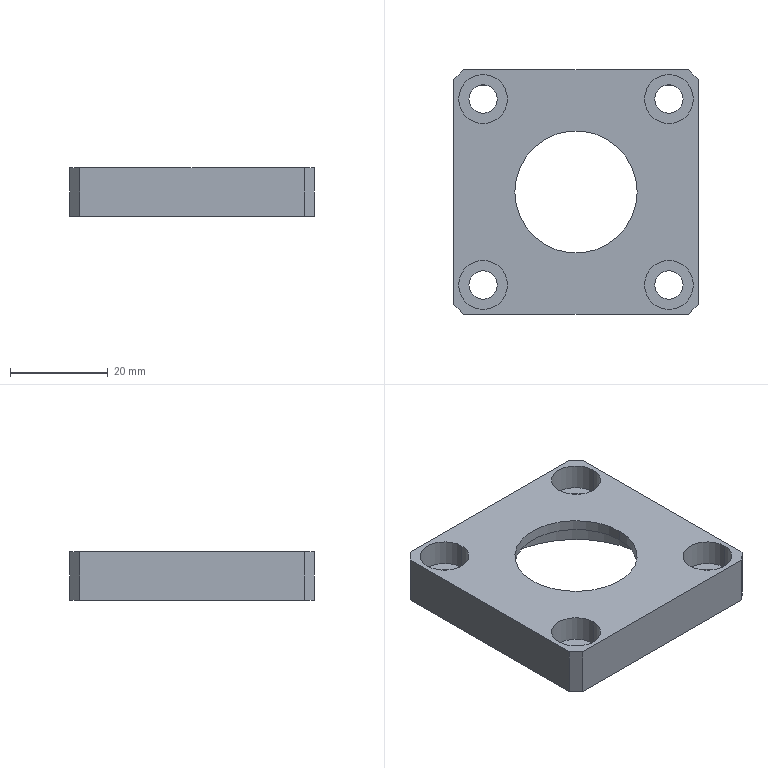Part | SolidWorks | features ICE 2, Chamfer 1, Extrusion 1, HoleWzd 1 | 1 solid | 35 faces | box 50 x 50 x 10 mm | volume 11856 mm3 | cylinder 20 | plane 15 | commonest cylinder face diameters 5.8 x8 10 x8 25 x2 40 x2
STEP:
#1=CARTESIAN_POINT('',(-12.5,0.,2.8));
#2=VERTEX_POINT('',#1);
#3=CARTESIAN_POINT('',(12.5,0.,2.8));
#4=VERTEX_POINT('',#3);
#5=CARTESIAN_POINT('',(0.,0.,2.8));
#6=DIRECTION('',(0.,0.,1.));
#7=DIRECTION('',(1.,0.,0.));
#8=AXIS2_PLACEMENT_3D('',#5,#6,#7);
#9=CIRCLE('',#8,12.5);
#10=EDGE_CURVE('',#2,#4,#9,.T.);
#11=ORIENTED_EDGE('',*,*,#10,.F.);
#12=CARTESIAN_POINT('',(-12.5,0.,5.));
#13=VERTEX_POINT('',#12);
#14=CARTESIAN_POINT('',(-12.5,0.,2.8));
#15=DIRECTION('',(0.,0.,1.));
#16=VECTOR('',#15,1000.);
#17=LINE('',#14,#16);
#18=EDGE_CURVE('',#2,#13,#17,.T.);
#19=ORIENTED_EDGE('',*,*,#18,.T.);
#20=CARTESIAN_POINT('',(12.5,0.,5.));
#21=VERTEX_POINT('',#20);
#22=CARTESIAN_POINT('',(0.,0.,5.));
#23=DIRECTION('',(0.,0.,1.));
#24=DIRECTION('',(1.,0.,0.));
#25=AXIS2_PLACEMENT_3D('',#22,#23,#24);
#26=CIRCLE('',#25,12.5);
#27=EDGE_CURVE('',#13,#21,#26,.T.);
#28=ORIENTED_EDGE('',*,*,#27,.T.);
#29=CARTESIAN_POINT('',(12.5,0.,2.8));
#30=DIRECTION('',(0.,0.,1.));
#31=VECTOR('',#30,1000.);
#32=LINE('',#29,#31);
#33=EDGE_CURVE('',#4,#21,#32,.T.);
#34=ORIENTED_EDGE('',*,*,#33,.F.);
#35=EDGE_LOOP('',(#11,#19,#28,#34));
#36=FACE_OUTER_BOUND('',#35,.T.);
#37=CARTESIAN_POINT('',(0.,0.,2.8));
#38=DIRECTION('',(0.,0.,1.));
#39=DIRECTION('',(1.,0.,0.));
#40=AXIS2_PLACEMENT_3D('',#37,#38,#39);
#41=CYLINDRICAL_SURFACE('',#40,12.5);
#42=ADVANCED_FACE('',(#36),#41,.F.);
#43=CARTESIAN_POINT('',(-24.,19.,-0.4));
#44=VERTEX_POINT('',#43);
#45=CARTESIAN_POINT('',(-14.,19.,-0.4));
#46=VERTEX_POINT('',#45);
#47=CARTESIAN_POINT('',(-19.,19.,-0.4));
#48=DIRECTION('',(0.,0.,1.));
#49=DIRECTION('',(1.,0.,0.));
#50=AXIS2_PLACEMENT_3D('',#47,#48,#49);
#51=CIRCLE('',#50,5.);
#52=EDGE_CURVE('',#44,#46,#51,.T.);
#53=ORIENTED_EDGE('',*,*,#52,.F.);
#54=CARTESIAN_POINT('',(-24.,19.,5.));
#55=VERTEX_POINT('',#54);
#56=CARTESIAN_POINT('',(-24.,19.,5.));
#57=DIRECTION('',(0.,0.,1.));
#58=VECTOR('',#57,1000.);
#59=LINE('',#56,#58);
#60=EDGE_CURVE('',#44,#55,#59,.T.);
#61=ORIENTED_EDGE('',*,*,#60,.T.);
#62=CARTESIAN_POINT('',(-14.,19.,5.));
#63=VERTEX_POINT('',#62);
#64=CARTESIAN_POINT('',(-19.,19.,5.));
#65=DIRECTION('',(0.,0.,1.));
#66=DIRECTION('',(1.,0.,0.));
#67=AXIS2_PLACEMENT_3D('',#64,#65,#66);
#68=CIRCLE('',#67,5.);
#69=EDGE_CURVE('',#55,#63,#68,.T.);
#70=ORIENTED_EDGE('',*,*,#69,.T.);
#71=CARTESIAN_POINT('',(-14.,19.,5.));
#72=DIRECTION('',(0.,0.,1.));
#73=VECTOR('',#72,1000.);
#74=LINE('',#71,#73);
#75=EDGE_CURVE('',#46,#63,#74,.T.);
#76=ORIENTED_EDGE('',*,*,#75,.F.);
#77=EDGE_LOOP('',(#53,#61,#70,#76));
#78=FACE_OUTER_BOUND('',#77,.T.);
#79=CARTESIAN_POINT('',(-19.,19.,5.));
#80=DIRECTION('',(0.,0.,1.));
#81=DIRECTION('',(1.,0.,0.));
#82=AXIS2_PLACEMENT_3D('',#79,#80,#81);
#83=CYLINDRICAL_SURFACE('',#82,5.);
#84=ADVANCED_FACE('',(#78),#83,.F.);
#85=CARTESIAN_POINT('',(-21.9,19.,-5.));
#86=VERTEX_POINT('',#85);
#87=CARTESIAN_POINT('',(-16.1,19.,-5.));
#88=VERTEX_POINT('',#87);
#89=CARTESIAN_POINT('',(-19.,19.,-5.));
#90=DIRECTION('',(0.,0.,1.));
#91=DIRECTION('',(1.,0.,0.));
#92=AXIS2_PLACEMENT_3D('',#89,#90,#91);
#93=CIRCLE('',#92,2.9);
#94=EDGE_CURVE('',#86,#88,#93,.T.);
#95=ORIENTED_EDGE('',*,*,#94,.F.);
#96=CARTESIAN_POINT('',(-21.9,19.,-0.4));
#97=VERTEX_POINT('',#96);
#98=CARTESIAN_POINT('',(-21.9,19.,5.));
#99=DIRECTION('',(0.,0.,1.));
#100=VECTOR('',#99,1000.);
#101=LINE('',#98,#100);
#102=EDGE_CURVE('',#86,#97,#101,.T.);
#103=ORIENTED_EDGE('',*,*,#102,.T.);
#104=CARTESIAN_POINT('',(-16.1,19.,-0.4));
#105=VERTEX_POINT('',#104);
#106=CARTESIAN_POINT('',(-19.,19.,-0.4));
#107=DIRECTION('',(0.,0.,1.));
#108=DIRECTION('',(1.,0.,0.));
#109=AXIS2_PLACEMENT_3D('',#106,#107,#108);
#110=CIRCLE('',#109,2.9);
#111=EDGE_CURVE('',#97,#105,#110,.T.);
#112=ORIENTED_EDGE('',*,*,#111,.T.);
#113=CARTESIAN_POINT('',(-16.1,19.,5.));
#114=DIRECTION('',(0.,0.,1.));
#115=VECTOR('',#114,1000.);
#116=LINE('',#113,#115);
#117=EDGE_CURVE('',#88,#105,#116,.T.);
#118=ORIENTED_EDGE('',*,*,#117,.F.);
#119=EDGE_LOOP('',(#95,#103,#112,#118));
#120=FACE_OUTER_BOUND('',#119,.T.);
#121=CARTESIAN_POINT('',(-19.,19.,5.));
#122=DIRECTION('',(0.,0.,1.));
#123=DIRECTION('',(1.,0.,0.));
#124=AXIS2_PLACEMENT_3D('',#121,#122,#123);
#125=CYLINDRICAL_SURFACE('',#124,2.9);
#126=ADVANCED_FACE('',(#120),#125,.F.);
#127=CARTESIAN_POINT('',(14.,19.,-0.4));
#128=VERTEX_POINT('',#127);
#129=CARTESIAN_POINT('',(24.,19.,-0.4));
#130=VERTEX_POINT('',#129);
#131=CARTESIAN_POINT('',(19.,19.,-0.4));
#132=DIRECTION('',(0.,0.,1.));
#133=DIRECTION('',(1.,0.,0.));
#134=AXIS2_PLACEMENT_3D('',#131,#132,#133);
#135=CIRCLE('',#134,5.);
#136=EDGE_CURVE('',#128,#130,#135,.T.);
#137=ORIENTED_EDGE('',*,*,#136,.F.);
#138=CARTESIAN_POINT('',(14.,19.,5.));
#139=VERTEX_POINT('',#138);
#140=CARTESIAN_POINT('',(14.,19.,5.));
#141=DIRECTION('',(0.,0.,1.));
#142=VECTOR('',#141,1000.);
#143=LINE('',#140,#142);
#144=EDGE_CURVE('',#128,#139,#143,.T.);
#145=ORIENTED_EDGE('',*,*,#144,.T.);
#146=CARTESIAN_POINT('',(24.,19.,5.));
#147=VERTEX_POINT('',#146);
#148=CARTESIAN_POINT('',(19.,19.,5.));
#149=DIRECTION('',(0.,0.,1.));
#150=DIRECTION('',(1.,0.,0.));
#151=AXIS2_PLACEMENT_3D('',#148,#149,#150);
#152=CIRCLE('',#151,5.);
#153=EDGE_CURVE('',#139,#147,#152,.T.);
#154=ORIENTED_EDGE('',*,*,#153,.T.);
#155=CARTESIAN_POINT('',(24.,19.,5.));
#156=DIRECTION('',(0.,0.,1.));
#157=VECTOR('',#156,1000.);
#158=LINE('',#155,#157);
#159=EDGE_CURVE('',#130,#147,#158,.T.);
#160=ORIENTED_EDGE('',*,*,#159,.F.);
#161=EDGE_LOOP('',(#137,#145,#154,#160));
#162=FACE_OUTER_BOUND('',#161,.T.);
#163=CARTESIAN_POINT('',(19.,19.,5.));
#164=DIRECTION('',(0.,0.,1.));
#165=DIRECTION('',(1.,0.,0.));
#166=AXIS2_PLACEMENT_3D('',#163,#164,#165);
#167=CYLINDRICAL_SURFACE('',#166,5.);
#168=ADVANCED_FACE('',(#162),#167,.F.);
#169=CARTESIAN_POINT('',(16.1,19.,-5.));
#170=VERTEX_POINT('',#169);
#171=CARTESIAN_POINT('',(21.9,19.,-5.));
#172=VERTEX_POINT('',#171);
#173=CARTESIAN_POINT('',(19.,19.,-5.));
#174=DIRECTION('',(0.,0.,1.));
#175=DIRECTION('',(1.,0.,0.));
#176=AXIS2_PLACEMENT_3D('',#173,#174,#175);
#177=CIRCLE('',#176,2.9);
#178=EDGE_CURVE('',#170,#172,#177,.T.);
#179=ORIENTED_EDGE('',*,*,#178,.F.);
#180=CARTESIAN_POINT('',(16.1,19.,-0.4));
#181=VERTEX_POINT('',#180);
#182=CARTESIAN_POINT('',(16.1,19.,5.));
#183=DIRECTION('',(0.,0.,1.));
#184=VECTOR('',#183,1000.);
#185=LINE('',#182,#184);
#186=EDGE_CURVE('',#170,#181,#185,.T.);
#187=ORIENTED_EDGE('',*,*,#186,.T.);
#188=CARTESIAN_POINT('',(21.9,19.,-0.4));
#189=VERTEX_POINT('',#188);
#190=CARTESIAN_POINT('',(19.,19.,-0.4));
#191=DIRECTION('',(0.,0.,1.));
#192=DIRECTION('',(1.,0.,0.));
#193=AXIS2_PLACEMENT_3D('',#190,#191,#192);
#194=CIRCLE('',#193,2.9);
#195=EDGE_CURVE('',#181,#189,#194,.T.);
#196=ORIENTED_EDGE('',*,*,#195,.T.);
#197=CARTESIAN_POINT('',(21.9,19.,5.));
#198=DIRECTION('',(0.,0.,1.));
#199=VECTOR('',#198,1000.);
#200=LINE('',#197,#199);
#201=EDGE_CURVE('',#172,#189,#200,.T.);
#202=ORIENTED_EDGE('',*,*,#201,.F.);
#203=EDGE_LOOP('',(#179,#187,#196,#202));
#204=FACE_OUTER_BOUND('',#203,.T.);
#205=CARTESIAN_POINT('',(19.,19.,5.));
#206=DIRECTION('',(0.,0.,1.));
#207=DIRECTION('',(1.,0.,0.));
#208=AXIS2_PLACEMENT_3D('',#205,#206,#207);
#209=CYLINDRICAL_SURFACE('',#208,2.9);
#210=ADVANCED_FACE('',(#204),#209,.F.);
#211=CARTESIAN_POINT('',(-24.,-19.,-0.4));
#212=VERTEX_POINT('',#211);
#213=CARTESIAN_POINT('',(-14.,-19.,-0.4));
#214=VERTEX_POINT('',#213);
#215=CARTESIAN_POINT('',(-19.,-19.,-0.4));
#216=DIRECTION('',(0.,0.,1.));
#217=DIRECTION('',(1.,0.,0.));
#218=AXIS2_PLACEMENT_3D('',#215,#216,#217);
#219=CIRCLE('',#218,5.);
#220=EDGE_CURVE('',#212,#214,#219,.T.);
#221=ORIENTED_EDGE('',*,*,#220,.F.);
#222=CARTESIAN_POINT('',(-24.,-19.,5.));
#223=VERTEX_POINT('',#222);
#224=CARTESIAN_POINT('',(-24.,-19.,5.));
#225=DIRECTION('',(0.,0.,1.));
#226=VECTOR('',#225,1000.);
#227=LINE('',#224,#226);
#228=EDGE_CURVE('',#212,#223,#227,.T.);
#229=ORIENTED_EDGE('',*,*,#228,.T.);
#230=CARTESIAN_POINT('',(-14.,-19.,5.));
#231=VERTEX_POINT('',#230);
#232=CARTESIAN_POINT('',(-19.,-19.,5.));
#233=DIRECTION('',(0.,0.,1.));
#234=DIRECTION('',(1.,0.,0.));
#235=AXIS2_PLACEMENT_3D('',#232,#233,#234);
#236=CIRCLE('',#235,5.);
#237=EDGE_CURVE('',#223,#231,#236,.T.);
#238=ORIENTED_EDGE('',*,*,#237,.T.);
#239=CARTESIAN_POINT('',(-14.,-19.,5.));
#240=DIRECTION('',(0.,0.,1.));
#241=VECTOR('',#240,1000.);
#242=LINE('',#239,#241);
#243=EDGE_CURVE('',#214,#231,#242,.T.);
#244=ORIENTED_EDGE('',*,*,#243,.F.);
#245=EDGE_LOOP('',(#221,#229,#238,#244));
#246=FACE_OUTER_BOUND('',#245,.T.);
#247=CARTESIAN_POINT('',(-19.,-19.,5.));
#248=DIRECTION('',(0.,0.,1.));
#249=DIRECTION('',(1.,0.,0.));
#250=AXIS2_PLACEMENT_3D('',#247,#248,#249);
#251=CYLINDRICAL_SURFACE('',#250,5.);
#252=ADVANCED_FACE('',(#246),#251,.F.);
#253=CARTESIAN_POINT('',(-21.9,-19.,-5.));
#254=VERTEX_POINT('',#253);
#255=CARTESIAN_POINT('',(-16.1,-19.,-5.));
#256=VERTEX_POINT('',#255);
#257=CARTESIAN_POINT('',(-19.,-19.,-5.));
#258=DIRECTION('',(0.,0.,1.));
#259=DIRECTION('',(1.,0.,0.));
#260=AXIS2_PLACEMENT_3D('',#257,#258,#259);
#261=CIRCLE('',#260,2.9);
#262=EDGE_CURVE('',#254,#256,#261,.T.);
#263=ORIENTED_EDGE('',*,*,#262,.F.);
#264=CARTESIAN_POINT('',(-21.9,-19.,-0.4));
#265=VERTEX_POINT('',#264);
#266=CARTESIAN_POINT('',(-21.9,-19.,5.));
#267=DIRECTION('',(0.,0.,1.));
#268=VECTOR('',#267,1000.);
#269=LINE('',#266,#268);
#270=EDGE_CURVE('',#254,#265,#269,.T.);
#271=ORIENTED_EDGE('',*,*,#270,.T.);
#272=CARTESIAN_POINT('',(-16.1,-19.,-0.4));
#273=VERTEX_POINT('',#272);
#274=CARTESIAN_POINT('',(-19.,-19.,-0.4));
#275=DIRECTION('',(0.,0.,1.));
#276=DIRECTION('',(1.,0.,0.));
#277=AXIS2_PLACEMENT_3D('',#274,#275,#276);
#278=CIRCLE('',#277,2.9);
#279=EDGE_CURVE('',#265,#273,#278,.T.);
#280=ORIENTED_EDGE('',*,*,#279,.T.);
#281=CARTESIAN_POINT('',(-16.1,-19.,5.));
#282=DIRECTION('',(0.,0.,1.));
#283=VECTOR('',#282,1000.);
#284=LINE('',#281,#283);
#285=EDGE_CURVE('',#256,#273,#284,.T.);
#286=ORIENTED_EDGE('',*,*,#285,.F.);
#287=EDGE_LOOP('',(#263,#271,#280,#286));
#288=FACE_OUTER_BOUND('',#287,.T.);
#289=CARTESIAN_POINT('',(-19.,-19.,5.));
#290=DIRECTION('',(0.,0.,1.));
#291=DIRECTION('',(1.,0.,0.));
#292=AXIS2_PLACEMENT_3D('',#289,#290,#291);
#293=CYLINDRICAL_SURFACE('',#292,2.9);
#294=ADVANCED_FACE('',(#288),#293,.F.);
#295=CARTESIAN_POINT('',(14.,-19.,-0.4));
#296=VERTEX_POINT('',#295);
#297=CARTESIAN_POINT('',(24.,-19.,-0.4));
#298=VERTEX_POINT('',#297);
#299=CARTESIAN_POINT('',(19.,-19.,-0.4));
#300=DIRECTION('',(0.,0.,1.));
#301=DIRECTION('',(1.,0.,0.));
#302=AXIS2_PLACEMENT_3D('',#299,#300,#301);
#303=CIRCLE('',#302,5.);
#304=EDGE_CURVE('',#296,#298,#303,.T.);
#305=ORIENTED_EDGE('',*,*,#304,.F.);
#306=CARTESIAN_POINT('',(14.,-19.,5.));
#307=VERTEX_POINT('',#306);
#308=CARTESIAN_POINT('',(14.,-19.,5.));
#309=DIRECTION('',(0.,0.,1.));
#310=VECTOR('',#309,1000.);
#311=LINE('',#308,#310);
#312=EDGE_CURVE('',#296,#307,#311,.T.);
#313=ORIENTED_EDGE('',*,*,#312,.T.);
#314=CARTESIAN_POINT('',(24.,-19.,5.));
#315=VERTEX_POINT('',#314);
#316=CARTESIAN_POINT('',(19.,-19.,5.));
#317=DIRECTION('',(0.,0.,1.));
#318=DIRECTION('',(1.,0.,0.));
#319=AXIS2_PLACEMENT_3D('',#316,#317,#318);
#320=CIRCLE('',#319,5.);
#321=EDGE_CURVE('',#307,#315,#320,.T.);
#322=ORIENTED_EDGE('',*,*,#321,.T.);
#323=CARTESIAN_POINT('',(24.,-19.,5.));
#324=DIRECTION('',(0.,0.,1.));
#325=VECTOR('',#324,1000.);
#326=LINE('',#323,#325);
#327=EDGE_CURVE('',#298,#315,#326,.T.);
#328=ORIENTED_EDGE('',*,*,#327,.F.);
#329=EDGE_LOOP('',(#305,#313,#322,#328));
#330=FACE_OUTER_BOUND('',#329,.T.);
#331=CARTESIAN_POINT('',(19.,-19.,5.));
#332=DIRECTION('',(0.,0.,1.));
#333=DIRECTION('',(1.,0.,0.));
#334=AXIS2_PLACEMENT_3D('',#331,#332,#333);
#335=CYLINDRICAL_SURFACE('',#334,5.);
#336=ADVANCED_FACE('',(#330),#335,.F.);
#337=CARTESIAN_POINT('',(16.1,-19.,-5.));
#338=VERTEX_POINT('',#337);
#339=CARTESIAN_POINT('',(21.9,-19.,-5.));
#340=VERTEX_POINT('',#339);
#341=CARTESIAN_POINT('',(19.,-19.,-5.));
#342=DIRECTION('',(0.,0.,1.));
#343=DIRECTION('',(1.,0.,0.));
#344=AXIS2_PLACEMENT_3D('',#341,#342,#343);
#345=CIRCLE('',#344,2.9);
#346=EDGE_CURVE('',#338,#340,#345,.T.);
#347=ORIENTED_EDGE('',*,*,#346,.F.);
#348=CARTESIAN_POINT('',(16.1,-19.,-0.4));
#349=VERTEX_POINT('',#348);
#350=CARTESIAN_POINT('',(16.1,-19.,5.));
#351=DIRECTION('',(0.,0.,1.));
#352=VECTOR('',#351,1000.);
#353=LINE('',#350,#352);
#354=EDGE_CURVE('',#338,#349,#353,.T.);
#355=ORIENTED_EDGE('',*,*,#354,.T.);
#356=CARTESIAN_POINT('',(21.9,-19.,-0.4));
#357=VERTEX_POINT('',#356);
#358=CARTESIAN_POINT('',(19.,-19.,-0.4));
#359=DIRECTION('',(0.,0.,1.));
#360=DIRECTION('',(1.,0.,0.));
#361=AXIS2_PLACEMENT_3D('',#358,#359,#360);
#362=CIRCLE('',#361,2.9);
#363=EDGE_CURVE('',#349,#357,#362,.T.);
#364=ORIENTED_EDGE('',*,*,#363,.T.);
#365=CARTESIAN_POINT('',(21.9,-19.,5.));
#366=DIRECTION('',(0.,0.,1.));
#367=VECTOR('',#366,1000.);
#368=LINE('',#365,#367);
#369=EDGE_CURVE('',#340,#357,#368,.T.);
#370=ORIENTED_EDGE('',*,*,#369,.F.);
#371=EDGE_LOOP('',(#347,#355,#364,#370));
#372=FACE_OUTER_BOUND('',#371,.T.);
#373=CARTESIAN_POINT('',(19.,-19.,5.));
#374=DIRECTION('',(0.,0.,1.));
#375=DIRECTION('',(1.,0.,0.));
#376=AXIS2_PLACEMENT_3D('',#373,#374,#375);
#377=CYLINDRICAL_SURFACE('',#376,2.9);
#378=ADVANCED_FACE('',(#372),#377,.F.);
#379=CARTESIAN_POINT('',(-20.,0.,-5.));
#380=VERTEX_POINT('',#379);
#381=CARTESIAN_POINT('',(20.,0.,-5.));
#382=VERTEX_POINT('',#381);
#383=CARTESIAN_POINT('',(0.,0.,-5.));
#384=DIRECTION('',(0.,0.,1.));
#385=DIRECTION('',(1.,0.,0.));
#386=AXIS2_PLACEMENT_3D('',#383,#384,#385);
#387=CIRCLE('',#386,20.);
#388=EDGE_CURVE('',#380,#382,#387,.T.);
#389=ORIENTED_EDGE('',*,*,#388,.F.);
#390=CARTESIAN_POINT('',(-20.,0.,2.8));
#391=VERTEX_POINT('',#390);
#392=CARTESIAN_POINT('',(-20.,0.,-5.));
#393=DIRECTION('',(0.,0.,1.));
#394=VECTOR('',#393,1000.);
#395=LINE('',#392,#394);
#396=EDGE_CURVE('',#380,#391,#395,.T.);
#397=ORIENTED_EDGE('',*,*,#396,.T.);
#398=CARTESIAN_POINT('',(20.,0.,2.8));
#399=VERTEX_POINT('',#398);
#400=CARTESIAN_POINT('',(0.,0.,2.8));
#401=DIRECTION('',(0.,0.,-1.));
#402=DIRECTION('',(1.,0.,0.));
#403=AXIS2_PLACEMENT_3D('',#400,#401,#402);
#404=CIRCLE('',#403,20.);
#405=EDGE_CURVE('',#399,#391,#404,.T.);
#406=ORIENTED_EDGE('',*,*,#405,.F.);
#407=CARTESIAN_POINT('',(20.,0.,-5.));
#408=DIRECTION('',(0.,0.,1.));
#409=VECTOR('',#408,1000.);
#410=LINE('',#407,#409);
#411=EDGE_CURVE('',#382,#399,#410,.T.);
#412=ORIENTED_EDGE('',*,*,#411,.F.);
#413=EDGE_LOOP('',(#389,#397,#406,#412));
#414=FACE_OUTER_BOUND('',#413,.T.);
#415=CARTESIAN_POINT('',(0.,0.,-5.));
#416=DIRECTION('',(0.,0.,1.));
#417=DIRECTION('',(1.,0.,0.));
#418=AXIS2_PLACEMENT_3D('',#415,#416,#417);
#419=CYLINDRICAL_SURFACE('',#418,20.);
#420=ADVANCED_FACE('',(#414),#419,.F.);
#421=ORIENTED_EDGE('',*,*,#396,.F.);
#422=CARTESIAN_POINT('',(0.,0.,-5.));
#423=DIRECTION('',(0.,0.,1.));
#424=DIRECTION('',(1.,0.,0.));
#425=AXIS2_PLACEMENT_3D('',#422,#423,#424);
#426=CIRCLE('',#425,20.);
#427=EDGE_CURVE('',#382,#380,#426,.T.);
#428=ORIENTED_EDGE('',*,*,#427,.F.);
#429=ORIENTED_EDGE('',*,*,#411,.T.);
#430=CARTESIAN_POINT('',(0.,0.,2.8));
#431=DIRECTION('',(0.,0.,-1.));
#432=DIRECTION('',(1.,0.,0.));
#433=AXIS2_PLACEMENT_3D('',#430,#431,#432);
#434=CIRCLE('',#433,20.);
#435=EDGE_CURVE('',#391,#399,#434,.T.);
#436=ORIENTED_EDGE('',*,*,#435,.F.);
#437=EDGE_LOOP('',(#421,#428,#429,#436));
#438=FACE_OUTER_BOUND('',#437,.T.);
#439=CARTESIAN_POINT('',(0.,0.,-5.));
#440=DIRECTION('',(0.,0.,1.));
#441=DIRECTION('',(1.,0.,0.));
#442=AXIS2_PLACEMENT_3D('',#439,#440,#441);
#443=CYLINDRICAL_SURFACE('',#442,20.);
#444=ADVANCED_FACE('',(#438),#443,.F.);
#445=CARTESIAN_POINT('',(25.,-23.,5.));
#446=VERTEX_POINT('',#445);
#447=CARTESIAN_POINT('',(25.,23.,5.));
#448=VERTEX_POINT('',#447);
#449=CARTESIAN_POINT('',(25.,-25.,5.));
#450=DIRECTION('',(0.,1.,0.));
#451=VECTOR('',#450,1000.);
#452=LINE('',#449,#451);
#453=EDGE_CURVE('',#446,#448,#452,.T.);
#454=ORIENTED_EDGE('',*,*,#453,.F.);
#455=CARTESIAN_POINT('',(25.,-23.,-5.));
#456=VERTEX_POINT('',#455);
#457=CARTESIAN_POINT('',(25.,-23.,5.));
#458=DIRECTION('',(0.,0.,-1.));
#459=VECTOR('',#458,1000.);
#460=LINE('',#457,#459);
#461=EDGE_CURVE('',#446,#456,#460,.T.);
#462=ORIENTED_EDGE('',*,*,#461,.T.);
#463=CARTESIAN_POINT('',(25.,23.,-5.));
#464=VERTEX_POINT('',#463);
#465=CARTESIAN_POINT('',(25.,-25.,-5.));
#466=DIRECTION('',(0.,1.,0.));
#467=VECTOR('',#466,1000.);
#468=LINE('',#465,#467);
#469=EDGE_CURVE('',#456,#464,#468,.T.);
#470=ORIENTED_EDGE('',*,*,#469,.T.);
#471=CARTESIAN_POINT('',(25.,23.,5.));
#472=DIRECTION('',(0.,0.,1.));
#473=VECTOR('',#472,1000.);
#474=LINE('',#471,#473);
#475=EDGE_CURVE('',#464,#448,#474,.T.);
#476=ORIENTED_EDGE('',*,*,#475,.T.);
#477=EDGE_LOOP('',(#454,#462,#470,#476));
#478=FACE_OUTER_BOUND('',#477,.T.);
#479=CARTESIAN_POINT('',(25.,-25.,5.));
#480=DIRECTION('',(-1.,0.,0.));
#481=DIRECTION('',(0.,0.,1.));
#482=AXIS2_PLACEMENT_3D('',#479,#480,#481);
#483=PLANE('',#482);
#484=ADVANCED_FACE('',(#478),#483,.F.);
#485=CARTESIAN_POINT('',(23.,25.,5.));
#486=VERTEX_POINT('',#485);
#487=CARTESIAN_POINT('',(-23.,25.,5.));
#488=VERTEX_POINT('',#487);
#489=CARTESIAN_POINT('',(-25.,25.,5.));
#490=DIRECTION('',(-1.,0.,0.));
#491=VECTOR('',#490,1000.);
#492=LINE('',#489,#491);
#493=EDGE_CURVE('',#486,#488,#492,.T.);
#494=ORIENTED_EDGE('',*,*,#493,.F.);
#495=CARTESIAN_POINT('',(23.,25.,-5.));
#496=VERTEX_POINT('',#495);
#497=CARTESIAN_POINT('',(23.,25.,5.));
#498=DIRECTION('',(0.,0.,-1.));
#499=VECTOR('',#498,1000.);
#500=LINE('',#497,#499);
#501=EDGE_CURVE('',#486,#496,#500,.T.);
#502=ORIENTED_EDGE('',*,*,#501,.T.);
#503=CARTESIAN_POINT('',(-23.,25.,-5.));
#504=VERTEX_POINT('',#503);
#505=CARTESIAN_POINT('',(-25.,25.,-5.));
#506=DIRECTION('',(-1.,0.,0.));
#507=VECTOR('',#506,1000.);
#508=LINE('',#505,#507);
#509=EDGE_CURVE('',#496,#504,#508,.T.);
#510=ORIENTED_EDGE('',*,*,#509,.T.);
#511=CARTESIAN_POINT('',(-23.,25.,5.));
#512=DIRECTION('',(0.,0.,1.));
#513=VECTOR('',#512,1000.);
#514=LINE('',#511,#513);
#515=EDGE_CURVE('',#504,#488,#514,.T.);
#516=ORIENTED_EDGE('',*,*,#515,.T.);
#517=EDGE_LOOP('',(#494,#502,#510,#516));
#518=FACE_OUTER_BOUND('',#517,.T.);
#519=CARTESIAN_POINT('',(-25.,25.,5.));
#520=DIRECTION('',(0.,-1.,0.));
#521=DIRECTION('',(0.,0.,-1.));
#522=AXIS2_PLACEMENT_3D('',#519,#520,#521);
#523=PLANE('',#522);
#524=ADVANCED_FACE('',(#518),#523,.F.);
#525=CARTESIAN_POINT('',(-25.,23.,-5.));
#526=VERTEX_POINT('',#525);
#527=CARTESIAN_POINT('',(-25.,-23.,-5.));
#528=VERTEX_POINT('',#527);
#529=CARTESIAN_POINT('',(-25.,-25.,-5.));
#530=DIRECTION('',(0.,-1.,0.));
#531=VECTOR('',#530,1000.);
#532=LINE('',#529,#531);
#533=EDGE_CURVE('',#526,#528,#532,.T.);
#534=ORIENTED_EDGE('',*,*,#533,.T.);
#535=CARTESIAN_POINT('',(-25.,-23.,5.));
#536=VERTEX_POINT('',#535);
#537=CARTESIAN_POINT('',(-25.,-23.,5.));
#538=DIRECTION('',(0.,0.,1.));
#539=VECTOR('',#538,1000.);
#540=LINE('',#537,#539);
#541=EDGE_CURVE('',#528,#536,#540,.T.);
#542=ORIENTED_EDGE('',*,*,#541,.T.);
#543=CARTESIAN_POINT('',(-25.,23.,5.));
#544=VERTEX_POINT('',#543);
#545=CARTESIAN_POINT('',(-25.,-25.,5.));
#546=DIRECTION('',(0.,-1.,0.));
#547=VECTOR('',#546,1000.);
#548=LINE('',#545,#547);
#549=EDGE_CURVE('',#544,#536,#548,.T.);
#550=ORIENTED_EDGE('',*,*,#549,.F.);
#551=CARTESIAN_POINT('',(-25.,23.,5.));
#552=DIRECTION('',(0.,0.,-1.));
#553=VECTOR('',#552,1000.);
#554=LINE('',#551,#553);
#555=EDGE_CURVE('',#544,#526,#554,.T.);
#556=ORIENTED_EDGE('',*,*,#555,.T.);
#557=EDGE_LOOP('',(#534,#542,#550,#556));
#558=FACE_OUTER_BOUND('',#557,.T.);
#559=CARTESIAN_POINT('',(-25.,-25.,5.));
#560=DIRECTION('',(1.,0.,0.));
#561=DIRECTION('',(0.,0.,-1.));
#562=AXIS2_PLACEMENT_3D('',#559,#560,#561);
#563=PLANE('',#562);
#564=ADVANCED_FACE('',(#558),#563,.F.);
#565=CARTESIAN_POINT('',(-23.,-25.,5.));
#566=VERTEX_POINT('',#565);
#567=CARTESIAN_POINT('',(23.,-25.,5.));
#568=VERTEX_POINT('',#567);
#569=CARTESIAN_POINT('',(-25.,-25.,5.));
#570=DIRECTION('',(1.,0.,0.));
#571=VECTOR('',#570,1000.);
#572=LINE('',#569,#571);
#573=EDGE_CURVE('',#566,#568,#572,.T.);
#574=ORIENTED_EDGE('',*,*,#573,.F.);
#575=CARTESIAN_POINT('',(-23.,-25.,-5.));
#576=VERTEX_POINT('',#575);
#577=CARTESIAN_POINT('',(-23.,-25.,5.));
#578=DIRECTION('',(0.,0.,-1.));
#579=VECTOR('',#578,1000.);
#580=LINE('',#577,#579);
#581=EDGE_CURVE('',#566,#576,#580,.T.);
#582=ORIENTED_EDGE('',*,*,#581,.T.);
#583=CARTESIAN_POINT('',(23.,-25.,-5.));
#584=VERTEX_POINT('',#583);
#585=CARTESIAN_POINT('',(-25.,-25.,-5.));
#586=DIRECTION('',(1.,0.,0.));
#587=VECTOR('',#586,1000.);
#588=LINE('',#585,#587);
#589=EDGE_CURVE('',#576,#584,#588,.T.);
#590=ORIENTED_EDGE('',*,*,#589,.T.);
#591=CARTESIAN_POINT('',(23.,-25.,5.));
#592=DIRECTION('',(0.,0.,1.));
#593=VECTOR('',#592,1000.);
#594=LINE('',#591,#593);
#595=EDGE_CURVE('',#584,#568,#594,.T.);
#596=ORIENTED_EDGE('',*,*,#595,.T.);
#597=EDGE_LOOP('',(#574,#582,#590,#596));
#598=FACE_OUTER_BOUND('',#597,.T.);
#599=CARTESIAN_POINT('',(-25.,-25.,5.));
#600=DIRECTION('',(0.,1.,0.));
#601=DIRECTION('',(0.,0.,1.));
#602=AXIS2_PLACEMENT_3D('',#599,#600,#601);
#603=PLANE('',#602);
#604=ADVANCED_FACE('',(#598),#603,.F.);
#605=CARTESIAN_POINT('',(-19.,19.,5.));
#606=DIRECTION('',(0.,0.,1.));
#607=DIRECTION('',(1.,0.,0.));
#608=AXIS2_PLACEMENT_3D('',#605,#606,#607);
#609=CIRCLE('',#608,5.);
#610=EDGE_CURVE('',#63,#55,#609,.T.);
#611=ORIENTED_EDGE('',*,*,#610,.F.);
#612=ORIENTED_EDGE('',*,*,#69,.F.);
#613=EDGE_LOOP('',(#611,#612));
#614=FACE_BOUND('',#613,.T.);
#615=CARTESIAN_POINT('',(19.,19.,5.));
#616=DIRECTION('',(0.,0.,1.));
#617=DIRECTION('',(1.,0.,0.));
#618=AXIS2_PLACEMENT_3D('',#615,#616,#617);
#619=CIRCLE('',#618,5.);
#620=EDGE_CURVE('',#147,#139,#619,.T.);
#621=ORIENTED_EDGE('',*,*,#620,.F.);
#622=ORIENTED_EDGE('',*,*,#153,.F.);
#623=EDGE_LOOP('',(#621,#622));
#624=FACE_BOUND('',#623,.T.);
#625=CARTESIAN_POINT('',(-19.,-19.,5.));
#626=DIRECTION('',(0.,0.,1.));
#627=DIRECTION('',(1.,0.,0.));
#628=AXIS2_PLACEMENT_3D('',#625,#626,#627);
#629=CIRCLE('',#628,5.);
#630=EDGE_CURVE('',#231,#223,#629,.T.);
#631=ORIENTED_EDGE('',*,*,#630,.F.);
#632=ORIENTED_EDGE('',*,*,#237,.F.);
#633=EDGE_LOOP('',(#631,#632));
#634=FACE_BOUND('',#633,.T.);
#635=CARTESIAN_POINT('',(19.,-19.,5.));
#636=DIRECTION('',(0.,0.,1.));
#637=DIRECTION('',(1.,0.,0.));
#638=AXIS2_PLACEMENT_3D('',#635,#636,#637);
#639=CIRCLE('',#638,5.);
#640=EDGE_CURVE('',#315,#307,#639,.T.);
#641=ORIENTED_EDGE('',*,*,#640,.F.);
#642=ORIENTED_EDGE('',*,*,#321,.F.);
#643=EDGE_LOOP('',(#641,#642));
#644=FACE_BOUND('',#643,.T.);
#645=ORIENTED_EDGE('',*,*,#549,.T.);
#646=CARTESIAN_POINT('',(-23.,-25.,5.));
#647=DIRECTION('',(0.7071,-0.7071,0.));
#648=VECTOR('',#647,1000.);
#649=LINE('',#646,#648);
#650=EDGE_CURVE('',#536,#566,#649,.T.);
#651=ORIENTED_EDGE('',*,*,#650,.T.);
#652=ORIENTED_EDGE('',*,*,#573,.T.);
#653=CARTESIAN_POINT('',(25.,-23.,5.));
#654=DIRECTION('',(0.7071,0.7071,0.));
#655=VECTOR('',#654,1000.);
#656=LINE('',#653,#655);
#657=EDGE_CURVE('',#568,#446,#656,.T.);
#658=ORIENTED_EDGE('',*,*,#657,.T.);
#659=ORIENTED_EDGE('',*,*,#453,.T.);
#660=CARTESIAN_POINT('',(23.,25.,5.));
#661=DIRECTION('',(-0.7071,0.7071,0.));
#662=VECTOR('',#661,1000.);
#663=LINE('',#660,#662);
#664=EDGE_CURVE('',#448,#486,#663,.T.);
#665=ORIENTED_EDGE('',*,*,#664,.T.);
#666=ORIENTED_EDGE('',*,*,#493,.T.);
#667=CARTESIAN_POINT('',(-25.,23.,5.));
#668=DIRECTION('',(-0.7071,-0.7071,0.));
#669=VECTOR('',#668,1000.);
#670=LINE('',#667,#669);
#671=EDGE_CURVE('',#488,#544,#670,.T.);
#672=ORIENTED_EDGE('',*,*,#671,.T.);
#673=EDGE_LOOP('',(#645,#651,#652,#658,#659,#665,#666,#672));
#674=FACE_OUTER_BOUND('',#673,.T.);
#675=CARTESIAN_POINT('',(0.,0.,5.));
#676=DIRECTION('',(0.,0.,1.));
#677=DIRECTION('',(1.,0.,0.));
#678=AXIS2_PLACEMENT_3D('',#675,#676,#677);
#679=CIRCLE('',#678,12.5);
#680=EDGE_CURVE('',#21,#13,#679,.T.);
#681=ORIENTED_EDGE('',*,*,#680,.F.);
#682=ORIENTED_EDGE('',*,*,#27,.F.);
#683=EDGE_LOOP('',(#681,#682));
#684=FACE_BOUND('',#683,.T.);
#685=CARTESIAN_POINT('',(0.,0.,5.));
#686=DIRECTION('',(0.,0.,-1.));
#687=DIRECTION('',(-1.,0.,0.));
#688=AXIS2_PLACEMENT_3D('',#685,#686,#687);
#689=PLANE('',#688);
#690=ADVANCED_FACE('',(#614,#624,#634,#644,#674,#684),#689,.F.);
#691=CARTESIAN_POINT('',(-19.,19.,-5.));
#692=DIRECTION('',(0.,0.,1.));
#693=DIRECTION('',(1.,0.,0.));
#694=AXIS2_PLACEMENT_3D('',#691,#692,#693);
#695=CIRCLE('',#694,2.9);
#696=EDGE_CURVE('',#88,#86,#695,.T.);
#697=ORIENTED_EDGE('',*,*,#696,.T.);
#698=ORIENTED_EDGE('',*,*,#94,.T.);
#699=EDGE_LOOP('',(#697,#698));
#700=FACE_BOUND('',#699,.T.);
#701=CARTESIAN_POINT('',(19.,19.,-5.));
#702=DIRECTION('',(0.,0.,1.));
#703=DIRECTION('',(1.,0.,0.));
#704=AXIS2_PLACEMENT_3D('',#701,#702,#703);
#705=CIRCLE('',#704,2.9);
#706=EDGE_CURVE('',#172,#170,#705,.T.);
#707=ORIENTED_EDGE('',*,*,#706,.T.);
#708=ORIENTED_EDGE('',*,*,#178,.T.);
#709=EDGE_LOOP('',(#707,#708));
#710=FACE_BOUND('',#709,.T.);
#711=CARTESIAN_POINT('',(-19.,-19.,-5.));
#712=DIRECTION('',(0.,0.,1.));
#713=DIRECTION('',(1.,0.,0.));
#714=AXIS2_PLACEMENT_3D('',#711,#712,#713);
#715=CIRCLE('',#714,2.9);
#716=EDGE_CURVE('',#256,#254,#715,.T.);
#717=ORIENTED_EDGE('',*,*,#716,.T.);
#718=ORIENTED_EDGE('',*,*,#262,.T.);
#719=EDGE_LOOP('',(#717,#718));
#720=FACE_BOUND('',#719,.T.);
#721=CARTESIAN_POINT('',(19.,-19.,-5.));
#722=DIRECTION('',(0.,0.,1.));
#723=DIRECTION('',(1.,0.,0.));
#724=AXIS2_PLACEMENT_3D('',#721,#722,#723);
#725=CIRCLE('',#724,2.9);
#726=EDGE_CURVE('',#340,#338,#725,.T.);
#727=ORIENTED_EDGE('',*,*,#726,.T.);
#728=ORIENTED_EDGE('',*,*,#346,.T.);
#729=EDGE_LOOP('',(#727,#728));
#730=FACE_BOUND('',#729,.T.);
#731=ORIENTED_EDGE('',*,*,#427,.T.);
#732=ORIENTED_EDGE('',*,*,#388,.T.);
#733=EDGE_LOOP('',(#731,#732));
#734=FACE_BOUND('',#733,.T.);
#735=ORIENTED_EDGE('',*,*,#589,.F.);
#736=CARTESIAN_POINT('',(-24.,-24.,-5.));
#737=DIRECTION('',(-0.7071,0.7071,0.));
#738=VECTOR('',#737,1000.);
#739=LINE('',#736,#738);
#740=EDGE_CURVE('',#576,#528,#739,.T.);
#741=ORIENTED_EDGE('',*,*,#740,.T.);
#742=ORIENTED_EDGE('',*,*,#533,.F.);
#743=CARTESIAN_POINT('',(-24.,24.,-5.));
#744=DIRECTION('',(0.7071,0.7071,0.));
#745=VECTOR('',#744,1000.);
#746=LINE('',#743,#745);
#747=EDGE_CURVE('',#526,#504,#746,.T.);
#748=ORIENTED_EDGE('',*,*,#747,.T.);
#749=ORIENTED_EDGE('',*,*,#509,.F.);
#750=CARTESIAN_POINT('',(24.,24.,-5.));
#751=DIRECTION('',(0.7071,-0.7071,0.));
#752=VECTOR('',#751,1000.);
#753=LINE('',#750,#752);
#754=EDGE_CURVE('',#496,#464,#753,.T.);
#755=ORIENTED_EDGE('',*,*,#754,.T.);
#756=ORIENTED_EDGE('',*,*,#469,.F.);
#757=CARTESIAN_POINT('',(24.,-24.,-5.));
#758=DIRECTION('',(-0.7071,-0.7071,0.));
#759=VECTOR('',#758,1000.);
#760=LINE('',#757,#759);
#761=EDGE_CURVE('',#456,#584,#760,.T.);
#762=ORIENTED_EDGE('',*,*,#761,.T.);
#763=EDGE_LOOP('',(#735,#741,#742,#748,#749,#755,#756,#762));
#764=FACE_OUTER_BOUND('',#763,.T.);
#765=CARTESIAN_POINT('',(0.,0.,-5.));
#766=DIRECTION('',(0.,0.,-1.));
#767=DIRECTION('',(-1.,0.,0.));
#768=AXIS2_PLACEMENT_3D('',#765,#766,#767);
#769=PLANE('',#768);
#770=ADVANCED_FACE('',(#700,#710,#720,#730,#734,#764),#769,.T.);
#771=ORIENTED_EDGE('',*,*,#354,.F.);
#772=ORIENTED_EDGE('',*,*,#726,.F.);
#773=ORIENTED_EDGE('',*,*,#369,.T.);
#774=CARTESIAN_POINT('',(19.,-19.,-0.4));
#775=DIRECTION('',(0.,0.,1.));
#776=DIRECTION('',(1.,0.,0.));
#777=AXIS2_PLACEMENT_3D('',#774,#775,#776);
#778=CIRCLE('',#777,2.9);
#779=EDGE_CURVE('',#357,#349,#778,.T.);
#780=ORIENTED_EDGE('',*,*,#779,.T.);
#781=EDGE_LOOP('',(#771,#772,#773,#780));
#782=FACE_OUTER_BOUND('',#781,.T.);
#783=CARTESIAN_POINT('',(19.,-19.,5.));
#784=DIRECTION('',(0.,0.,1.));
#785=DIRECTION('',(1.,0.,0.));
#786=AXIS2_PLACEMENT_3D('',#783,#784,#785);
#787=CYLINDRICAL_SURFACE('',#786,2.9);
#788=ADVANCED_FACE('',(#782),#787,.F.);
#789=ORIENTED_EDGE('',*,*,#779,.F.);
#790=ORIENTED_EDGE('',*,*,#363,.F.);
#791=EDGE_LOOP('',(#789,#790));
#792=FACE_BOUND('',#791,.T.);
#793=CARTESIAN_POINT('',(19.,-19.,-0.4));
#794=DIRECTION('',(0.,0.,1.));
#795=DIRECTION('',(1.,0.,0.));
#796=AXIS2_PLACEMENT_3D('',#793,#794,#795);
#797=CIRCLE('',#796,5.);
#798=EDGE_CURVE('',#298,#296,#797,.T.);
#799=ORIENTED_EDGE('',*,*,#798,.T.);
#800=ORIENTED_EDGE('',*,*,#304,.T.);
#801=EDGE_LOOP('',(#799,#800));
#802=FACE_OUTER_BOUND('',#801,.T.);
#803=CARTESIAN_POINT('',(21.9,-19.,-0.4));
#804=DIRECTION('',(0.,0.,-1.));
#805=DIRECTION('',(-1.,0.,0.));
#806=AXIS2_PLACEMENT_3D('',#803,#804,#805);
#807=PLANE('',#806);
#808=ADVANCED_FACE('',(#792,#802),#807,.F.);
#809=ORIENTED_EDGE('',*,*,#312,.F.);
#810=ORIENTED_EDGE('',*,*,#798,.F.);
#811=ORIENTED_EDGE('',*,*,#327,.T.);
#812=ORIENTED_EDGE('',*,*,#640,.T.);
#813=EDGE_LOOP('',(#809,#810,#811,#812));
#814=FACE_OUTER_BOUND('',#813,.T.);
#815=CARTESIAN_POINT('',(19.,-19.,5.));
#816=DIRECTION('',(0.,0.,1.));
#817=DIRECTION('',(1.,0.,0.));
#818=AXIS2_PLACEMENT_3D('',#815,#816,#817);
#819=CYLINDRICAL_SURFACE('',#818,5.);
#820=ADVANCED_FACE('',(#814),#819,.F.);
#821=ORIENTED_EDGE('',*,*,#270,.F.);
#822=ORIENTED_EDGE('',*,*,#716,.F.);
#823=ORIENTED_EDGE('',*,*,#285,.T.);
#824=CARTESIAN_POINT('',(-19.,-19.,-0.4));
#825=DIRECTION('',(0.,0.,1.));
#826=DIRECTION('',(1.,0.,0.));
#827=AXIS2_PLACEMENT_3D('',#824,#825,#826);
#828=CIRCLE('',#827,2.9);
#829=EDGE_CURVE('',#273,#265,#828,.T.);
#830=ORIENTED_EDGE('',*,*,#829,.T.);
#831=EDGE_LOOP('',(#821,#822,#823,#830));
#832=FACE_OUTER_BOUND('',#831,.T.);
#833=CARTESIAN_POINT('',(-19.,-19.,5.));
#834=DIRECTION('',(0.,0.,1.));
#835=DIRECTION('',(1.,0.,0.));
#836=AXIS2_PLACEMENT_3D('',#833,#834,#835);
#837=CYLINDRICAL_SURFACE('',#836,2.9);
#838=ADVANCED_FACE('',(#832),#837,.F.);
#839=ORIENTED_EDGE('',*,*,#829,.F.);
#840=ORIENTED_EDGE('',*,*,#279,.F.);
#841=EDGE_LOOP('',(#839,#840));
#842=FACE_BOUND('',#841,.T.);
#843=CARTESIAN_POINT('',(-19.,-19.,-0.4));
#844=DIRECTION('',(0.,0.,1.));
#845=DIRECTION('',(1.,0.,0.));
#846=AXIS2_PLACEMENT_3D('',#843,#844,#845);
#847=CIRCLE('',#846,5.);
#848=EDGE_CURVE('',#214,#212,#847,.T.);
#849=ORIENTED_EDGE('',*,*,#848,.T.);
#850=ORIENTED_EDGE('',*,*,#220,.T.);
#851=EDGE_LOOP('',(#849,#850));
#852=FACE_OUTER_BOUND('',#851,.T.);
#853=CARTESIAN_POINT('',(-16.1,-19.,-0.4));
#854=DIRECTION('',(0.,0.,-1.));
#855=DIRECTION('',(-1.,0.,0.));
#856=AXIS2_PLACEMENT_3D('',#853,#854,#855);
#857=PLANE('',#856);
#858=ADVANCED_FACE('',(#842,#852),#857,.F.);
#859=ORIENTED_EDGE('',*,*,#228,.F.);
#860=ORIENTED_EDGE('',*,*,#848,.F.);
#861=ORIENTED_EDGE('',*,*,#243,.T.);
#862=ORIENTED_EDGE('',*,*,#630,.T.);
#863=EDGE_LOOP('',(#859,#860,#861,#862));
#864=FACE_OUTER_BOUND('',#863,.T.);
#865=CARTESIAN_POINT('',(-19.,-19.,5.));
#866=DIRECTION('',(0.,0.,1.));
#867=DIRECTION('',(1.,0.,0.));
#868=AXIS2_PLACEMENT_3D('',#865,#866,#867);
#869=CYLINDRICAL_SURFACE('',#868,5.);
#870=ADVANCED_FACE('',(#864),#869,.F.);
#871=ORIENTED_EDGE('',*,*,#186,.F.);
#872=ORIENTED_EDGE('',*,*,#706,.F.);
#873=ORIENTED_EDGE('',*,*,#201,.T.);
#874=CARTESIAN_POINT('',(19.,19.,-0.4));
#875=DIRECTION('',(0.,0.,1.));
#876=DIRECTION('',(1.,0.,0.));
#877=AXIS2_PLACEMENT_3D('',#874,#875,#876);
#878=CIRCLE('',#877,2.9);
#879=EDGE_CURVE('',#189,#181,#878,.T.);
#880=ORIENTED_EDGE('',*,*,#879,.T.);
#881=EDGE_LOOP('',(#871,#872,#873,#880));
#882=FACE_OUTER_BOUND('',#881,.T.);
#883=CARTESIAN_POINT('',(19.,19.,5.));
#884=DIRECTION('',(0.,0.,1.));
#885=DIRECTION('',(1.,0.,0.));
#886=AXIS2_PLACEMENT_3D('',#883,#884,#885);
#887=CYLINDRICAL_SURFACE('',#886,2.9);
#888=ADVANCED_FACE('',(#882),#887,.F.);
#889=ORIENTED_EDGE('',*,*,#879,.F.);
#890=ORIENTED_EDGE('',*,*,#195,.F.);
#891=EDGE_LOOP('',(#889,#890));
#892=FACE_BOUND('',#891,.T.);
#893=CARTESIAN_POINT('',(19.,19.,-0.4));
#894=DIRECTION('',(0.,0.,1.));
#895=DIRECTION('',(1.,0.,0.));
#896=AXIS2_PLACEMENT_3D('',#893,#894,#895);
#897=CIRCLE('',#896,5.);
#898=EDGE_CURVE('',#130,#128,#897,.T.);
#899=ORIENTED_EDGE('',*,*,#898,.T.);
#900=ORIENTED_EDGE('',*,*,#136,.T.);
#901=EDGE_LOOP('',(#899,#900));
#902=FACE_OUTER_BOUND('',#901,.T.);
#903=CARTESIAN_POINT('',(21.9,19.,-0.4));
#904=DIRECTION('',(0.,0.,-1.));
#905=DIRECTION('',(-1.,0.,0.));
#906=AXIS2_PLACEMENT_3D('',#903,#904,#905);
#907=PLANE('',#906);
#908=ADVANCED_FACE('',(#892,#902),#907,.F.);
#909=ORIENTED_EDGE('',*,*,#144,.F.);
#910=ORIENTED_EDGE('',*,*,#898,.F.);
#911=ORIENTED_EDGE('',*,*,#159,.T.);
#912=ORIENTED_EDGE('',*,*,#620,.T.);
#913=EDGE_LOOP('',(#909,#910,#911,#912));
#914=FACE_OUTER_BOUND('',#913,.T.);
#915=CARTESIAN_POINT('',(19.,19.,5.));
#916=DIRECTION('',(0.,0.,1.));
#917=DIRECTION('',(1.,0.,0.));
#918=AXIS2_PLACEMENT_3D('',#915,#916,#917);
#919=CYLINDRICAL_SURFACE('',#918,5.);
#920=ADVANCED_FACE('',(#914),#919,.F.);
#921=ORIENTED_EDGE('',*,*,#102,.F.);
#922=ORIENTED_EDGE('',*,*,#696,.F.);
#923=ORIENTED_EDGE('',*,*,#117,.T.);
#924=CARTESIAN_POINT('',(-19.,19.,-0.4));
#925=DIRECTION('',(0.,0.,1.));
#926=DIRECTION('',(1.,0.,0.));
#927=AXIS2_PLACEMENT_3D('',#924,#925,#926);
#928=CIRCLE('',#927,2.9);
#929=EDGE_CURVE('',#105,#97,#928,.T.);
#930=ORIENTED_EDGE('',*,*,#929,.T.);
#931=EDGE_LOOP('',(#921,#922,#923,#930));
#932=FACE_OUTER_BOUND('',#931,.T.);
#933=CARTESIAN_POINT('',(-19.,19.,5.));
#934=DIRECTION('',(0.,0.,1.));
#935=DIRECTION('',(1.,0.,0.));
#936=AXIS2_PLACEMENT_3D('',#933,#934,#935);
#937=CYLINDRICAL_SURFACE('',#936,2.9);
#938=ADVANCED_FACE('',(#932),#937,.F.);
#939=ORIENTED_EDGE('',*,*,#929,.F.);
#940=ORIENTED_EDGE('',*,*,#111,.F.);
#941=EDGE_LOOP('',(#939,#940));
#942=FACE_BOUND('',#941,.T.);
#943=CARTESIAN_POINT('',(-19.,19.,-0.4));
#944=DIRECTION('',(0.,0.,1.));
#945=DIRECTION('',(1.,0.,0.));
#946=AXIS2_PLACEMENT_3D('',#943,#944,#945);
#947=CIRCLE('',#946,5.);
#948=EDGE_CURVE('',#46,#44,#947,.T.);
#949=ORIENTED_EDGE('',*,*,#948,.T.);
#950=ORIENTED_EDGE('',*,*,#52,.T.);
#951=EDGE_LOOP('',(#949,#950));
#952=FACE_OUTER_BOUND('',#951,.T.);
#953=CARTESIAN_POINT('',(-16.1,19.,-0.4));
#954=DIRECTION('',(0.,0.,-1.));
#955=DIRECTION('',(-1.,0.,0.));
#956=AXIS2_PLACEMENT_3D('',#953,#954,#955);
#957=PLANE('',#956);
#958=ADVANCED_FACE('',(#942,#952),#957,.F.);
#959=ORIENTED_EDGE('',*,*,#60,.F.);
#960=ORIENTED_EDGE('',*,*,#948,.F.);
#961=ORIENTED_EDGE('',*,*,#75,.T.);
#962=ORIENTED_EDGE('',*,*,#610,.T.);
#963=EDGE_LOOP('',(#959,#960,#961,#962));
#964=FACE_OUTER_BOUND('',#963,.T.);
#965=CARTESIAN_POINT('',(-19.,19.,5.));
#966=DIRECTION('',(0.,0.,1.));
#967=DIRECTION('',(1.,0.,0.));
#968=AXIS2_PLACEMENT_3D('',#965,#966,#967);
#969=CYLINDRICAL_SURFACE('',#968,5.);
#970=ADVANCED_FACE('',(#964),#969,.F.);
#971=ORIENTED_EDGE('',*,*,#650,.F.);
#972=ORIENTED_EDGE('',*,*,#541,.F.);
#973=ORIENTED_EDGE('',*,*,#740,.F.);
#974=ORIENTED_EDGE('',*,*,#581,.F.);
#975=EDGE_LOOP('',(#971,#972,#973,#974));
#976=FACE_OUTER_BOUND('',#975,.T.);
#977=CARTESIAN_POINT('',(-23.,-25.,5.));
#978=DIRECTION('',(0.7071,0.7071,0.));
#979=DIRECTION('',(0.,0.,-1.));
#980=AXIS2_PLACEMENT_3D('',#977,#978,#979);
#981=PLANE('',#980);
#982=ADVANCED_FACE('',(#976),#981,.F.);
#983=ORIENTED_EDGE('',*,*,#657,.F.);
#984=ORIENTED_EDGE('',*,*,#595,.F.);
#985=ORIENTED_EDGE('',*,*,#761,.F.);
#986=ORIENTED_EDGE('',*,*,#461,.F.);
#987=EDGE_LOOP('',(#983,#984,#985,#986));
#988=FACE_OUTER_BOUND('',#987,.T.);
#989=CARTESIAN_POINT('',(25.,-23.,5.));
#990=DIRECTION('',(-0.7071,0.7071,0.));
#991=DIRECTION('',(0.,0.,-1.));
#992=AXIS2_PLACEMENT_3D('',#989,#990,#991);
#993=PLANE('',#992);
#994=ADVANCED_FACE('',(#988),#993,.F.);
#995=ORIENTED_EDGE('',*,*,#664,.F.);
#996=ORIENTED_EDGE('',*,*,#475,.F.);
#997=ORIENTED_EDGE('',*,*,#754,.F.);
#998=ORIENTED_EDGE('',*,*,#501,.F.);
#999=EDGE_LOOP('',(#995,#996,#997,#998));
#1000=FACE_OUTER_BOUND('',#999,.T.);
#1001=CARTESIAN_POINT('',(23.,25.,5.));
#1002=DIRECTION('',(-0.7071,-0.7071,0.));
#1003=DIRECTION('',(0.,0.,-1.));
#1004=AXIS2_PLACEMENT_3D('',#1001,#1002,#1003);
#1005=PLANE('',#1004);
#1006=ADVANCED_FACE('',(#1000),#1005,.F.);
#1007=ORIENTED_EDGE('',*,*,#671,.F.);
#1008=ORIENTED_EDGE('',*,*,#515,.F.);
#1009=ORIENTED_EDGE('',*,*,#747,.F.);
#1010=ORIENTED_EDGE('',*,*,#555,.F.);
#1011=EDGE_LOOP('',(#1007,#1008,#1009,#1010));
#1012=FACE_OUTER_BOUND('',#1011,.T.);
#1013=CARTESIAN_POINT('',(-25.,23.,5.));
#1014=DIRECTION('',(0.7071,-0.7071,0.));
#1015=DIRECTION('',(0.,0.,-1.));
#1016=AXIS2_PLACEMENT_3D('',#1013,#1014,#1015);
#1017=PLANE('',#1016);
#1018=ADVANCED_FACE('',(#1012),#1017,.F.);
#1019=CARTESIAN_POINT('',(0.,0.,2.8));
#1020=DIRECTION('',(0.,0.,1.));
#1021=DIRECTION('',(1.,0.,0.));
#1022=AXIS2_PLACEMENT_3D('',#1019,#1020,#1021);
#1023=CIRCLE('',#1022,12.5);
#1024=EDGE_CURVE('',#4,#2,#1023,.T.);
#1025=ORIENTED_EDGE('',*,*,#1024,.T.);
#1026=ORIENTED_EDGE('',*,*,#10,.T.);
#1027=EDGE_LOOP('',(#1025,#1026));
#1028=FACE_BOUND('',#1027,.T.);
#1029=ORIENTED_EDGE('',*,*,#405,.T.);
#1030=ORIENTED_EDGE('',*,*,#435,.T.);
#1031=EDGE_LOOP('',(#1029,#1030));
#1032=FACE_OUTER_BOUND('',#1031,.T.);
#1033=CARTESIAN_POINT('',(0.,0.,2.8));
#1034=DIRECTION('',(0.,0.,1.));
#1035=DIRECTION('',(1.,0.,0.));
#1036=AXIS2_PLACEMENT_3D('',#1033,#1034,#1035);
#1037=PLANE('',#1036);
#1038=ADVANCED_FACE('',(#1028,#1032),#1037,.F.);
#1039=ORIENTED_EDGE('',*,*,#18,.F.);
#1040=ORIENTED_EDGE('',*,*,#1024,.F.);
#1041=ORIENTED_EDGE('',*,*,#33,.T.);
#1042=ORIENTED_EDGE('',*,*,#680,.T.);
#1043=EDGE_LOOP('',(#1039,#1040,#1041,#1042));
#1044=FACE_OUTER_BOUND('',#1043,.T.);
#1045=CARTESIAN_POINT('',(0.,0.,2.8));
#1046=DIRECTION('',(0.,0.,1.));
#1047=DIRECTION('',(1.,0.,0.));
#1048=AXIS2_PLACEMENT_3D('',#1045,#1046,#1047);
#1049=CYLINDRICAL_SURFACE('',#1048,12.5);
#1050=ADVANCED_FACE('',(#1044),#1049,.F.);
#1051=CLOSED_SHELL('',(#42,#84,#126,#168,#210,#252,#294,#336,#378,#420,#444,#484,#524,#564,#604,#690,#770,#788,#808,#820,#838,#858,#870,#888,#908,#920,#938,#958,#970,#982,#994,#1006,#1018,#1038,#1050));
#1052=MANIFOLD_SOLID_BREP('',#1051);
#1053=CARTESIAN_POINT('',(0.,0.,0.));
#1054=DIRECTION('',(0.,0.,1.));
#1055=DIRECTION('',(1.,0.,0.));
#1056=AXIS2_PLACEMENT_3D('',#1053,#1054,#1055);
#1057=(LENGTH_UNIT()NAMED_UNIT(*)SI_UNIT(.MILLI.,.METRE.));
#1058=UNCERTAINTY_MEASURE_WITH_UNIT(LENGTH_MEASURE(0.00001),#1057,'','');
#1059=(NAMED_UNIT(*)PLANE_ANGLE_UNIT()SI_UNIT($,.RADIAN.));
#1060=(NAMED_UNIT(*)SI_UNIT($,.STERADIAN.)SOLID_ANGLE_UNIT());
#1061=(GEOMETRIC_REPRESENTATION_CONTEXT(3)GLOBAL_UNCERTAINTY_ASSIGNED_CONTEXT((#1058))GLOBAL_UNIT_ASSIGNED_CONTEXT((#1057,#1059,#1060))REPRESENTATION_CONTEXT('',''));
#1062=ADVANCED_BREP_SHAPE_REPRESENTATION('',(#1052,#1056),#1061);